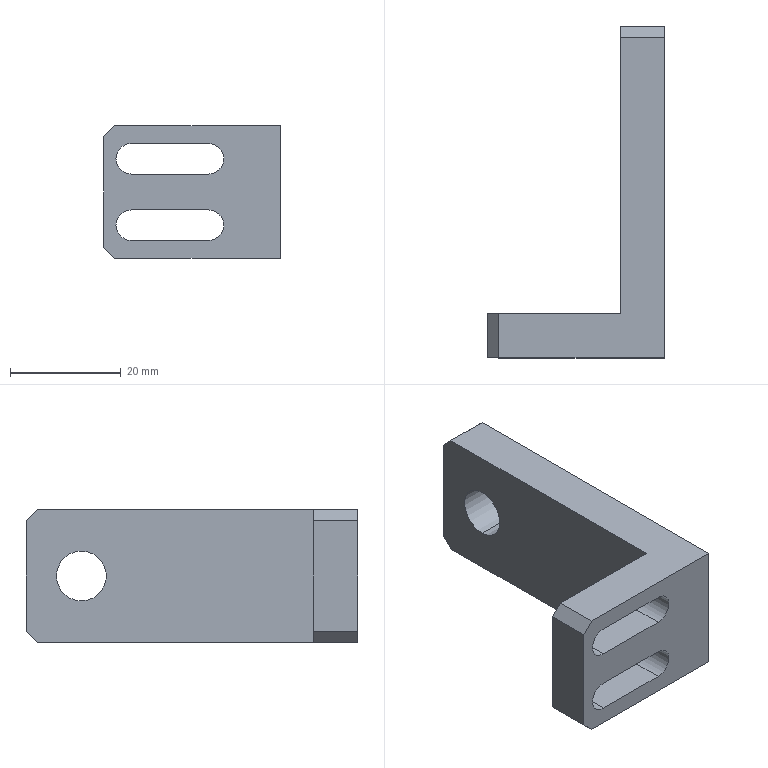Part | STEP file | 0-19 Buffer fixed | 1 solid | 24 faces | box 32 x 60 x 24 mm | volume 13943 mm3 | plane 16 | cylinder 8 | commonest cylinder face diameters 5.5 x6 9 x2